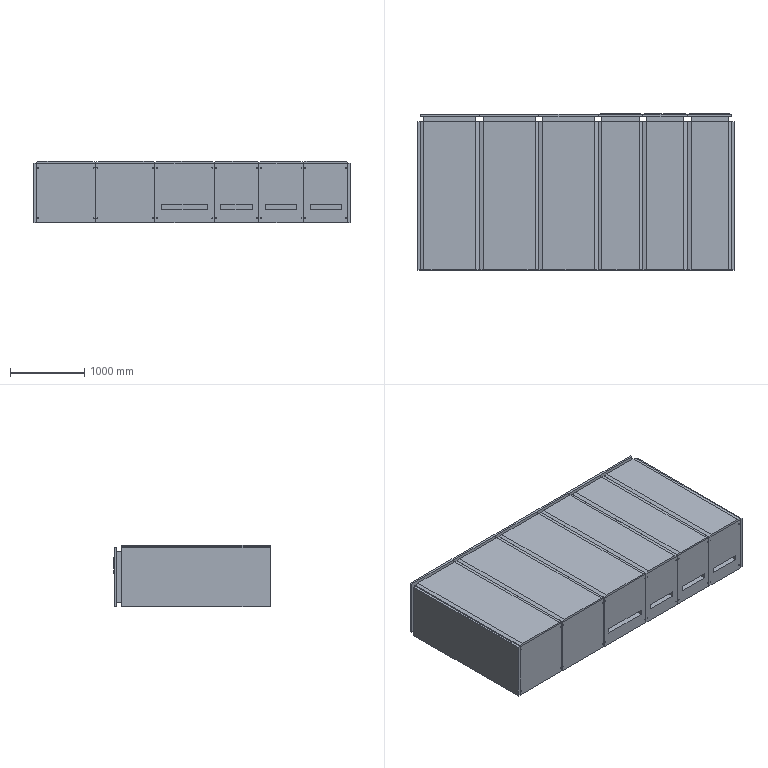Part | STEP file | 110VDC cabinet | 14 solids | 400 faces | box 4265 x 2106 x 827 mm | volume 7288083743 mm3 | plane 296 | spline 56 | cylinder 48 | commonest cylinder face diameters 11 x48